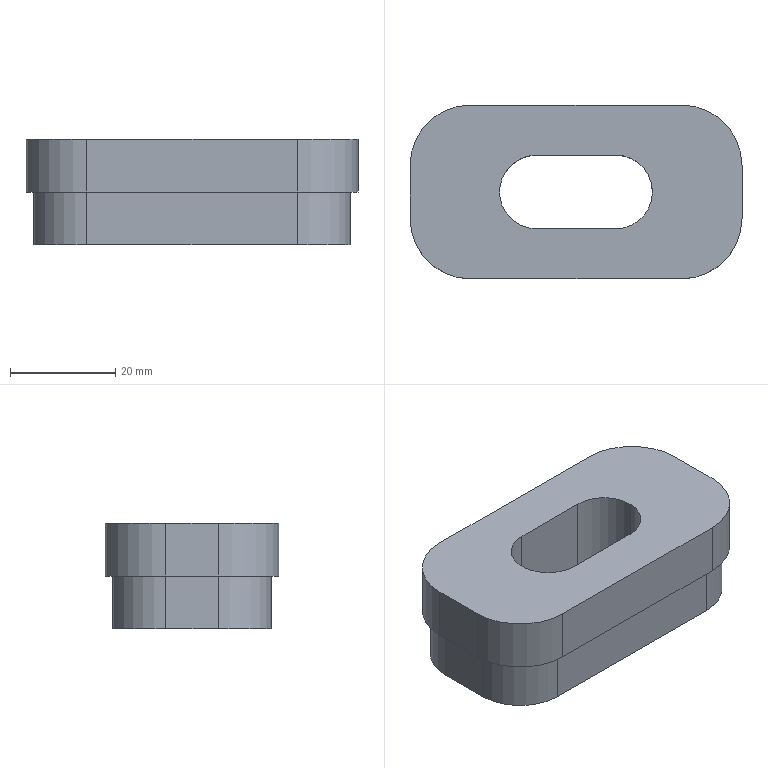Part | SolidWorks | features BaseBody 1 | 1 solid | 24 faces | box 63 x 33 x 20 mm | volume 29518 mm3 | plane 13 | cylinder 11 | commonest cylinder face diameters 20 x4 23 x4 14 x3
STEP:
#1=CARTESIAN_POINT('',(14.5,0.,0.));
#2=VERTEX_POINT('',#1);
#3=CARTESIAN_POINT('',(7.5,7.,0.));
#4=VERTEX_POINT('',#3);
#5=CARTESIAN_POINT('',(7.5,0.,0.));
#6=DIRECTION('',(0.,0.,1.));
#7=DIRECTION('',(1.,0.,0.));
#8=AXIS2_PLACEMENT_3D('',#5,#6,#7);
#9=CIRCLE('',#8,7.);
#10=EDGE_CURVE('',#2,#4,#9,.T.);
#11=ORIENTED_EDGE('',*,*,#10,.F.);
#12=CARTESIAN_POINT('',(14.5,0.,20.));
#13=VERTEX_POINT('',#12);
#14=CARTESIAN_POINT('',(14.5,0.,0.));
#15=DIRECTION('',(0.,0.,1.));
#16=VECTOR('',#15,1000.);
#17=LINE('',#14,#16);
#18=EDGE_CURVE('',#2,#13,#17,.T.);
#19=ORIENTED_EDGE('',*,*,#18,.T.);
#20=CARTESIAN_POINT('',(7.5,7.,20.));
#21=VERTEX_POINT('',#20);
#22=CARTESIAN_POINT('',(7.5,0.,20.));
#23=DIRECTION('',(0.,0.,-1.));
#24=DIRECTION('',(1.,0.,0.));
#25=AXIS2_PLACEMENT_3D('',#22,#23,#24);
#26=CIRCLE('',#25,7.);
#27=EDGE_CURVE('',#21,#13,#26,.T.);
#28=ORIENTED_EDGE('',*,*,#27,.F.);
#29=CARTESIAN_POINT('',(7.5,7.,0.));
#30=DIRECTION('',(0.,0.,1.));
#31=VECTOR('',#30,1000.);
#32=LINE('',#29,#31);
#33=EDGE_CURVE('',#4,#21,#32,.T.);
#34=ORIENTED_EDGE('',*,*,#33,.F.);
#35=EDGE_LOOP('',(#11,#19,#28,#34));
#36=FACE_OUTER_BOUND('',#35,.T.);
#37=CARTESIAN_POINT('',(7.5,0.,0.));
#38=DIRECTION('',(0.,0.,1.));
#39=DIRECTION('',(1.,0.,0.));
#40=AXIS2_PLACEMENT_3D('',#37,#38,#39);
#41=CYLINDRICAL_SURFACE('',#40,7.);
#42=ADVANCED_FACE('',(#36),#41,.F.);
#43=CARTESIAN_POINT('',(7.5,-7.,20.));
#44=VERTEX_POINT('',#43);
#45=CARTESIAN_POINT('',(-7.5,-7.,20.));
#46=VERTEX_POINT('',#45);
#47=CARTESIAN_POINT('',(0.,-7.,20.));
#48=DIRECTION('',(-1.,0.,0.));
#49=VECTOR('',#48,1000.);
#50=LINE('',#47,#49);
#51=EDGE_CURVE('',#44,#46,#50,.T.);
#52=ORIENTED_EDGE('',*,*,#51,.T.);
#53=CARTESIAN_POINT('',(-7.5,7.,20.));
#54=VERTEX_POINT('',#53);
#55=CARTESIAN_POINT('',(-7.5,0.,20.));
#56=DIRECTION('',(0.,0.,-1.));
#57=DIRECTION('',(1.,0.,0.));
#58=AXIS2_PLACEMENT_3D('',#55,#56,#57);
#59=CIRCLE('',#58,7.);
#60=EDGE_CURVE('',#46,#54,#59,.T.);
#61=ORIENTED_EDGE('',*,*,#60,.T.);
#62=CARTESIAN_POINT('',(0.,7.,20.));
#63=DIRECTION('',(1.,0.,0.));
#64=VECTOR('',#63,1000.);
#65=LINE('',#62,#64);
#66=EDGE_CURVE('',#54,#21,#65,.T.);
#67=ORIENTED_EDGE('',*,*,#66,.T.);
#68=ORIENTED_EDGE('',*,*,#27,.T.);
#69=CARTESIAN_POINT('',(7.5,0.,20.));
#70=DIRECTION('',(0.,0.,-1.));
#71=DIRECTION('',(1.,0.,0.));
#72=AXIS2_PLACEMENT_3D('',#69,#70,#71);
#73=CIRCLE('',#72,7.);
#74=EDGE_CURVE('',#13,#44,#73,.T.);
#75=ORIENTED_EDGE('',*,*,#74,.T.);
#76=EDGE_LOOP('',(#52,#61,#67,#68,#75));
#77=FACE_BOUND('',#76,.T.);
#78=CARTESIAN_POINT('',(31.5,-5.,20.));
#79=VERTEX_POINT('',#78);
#80=CARTESIAN_POINT('',(31.5,5.,20.));
#81=VERTEX_POINT('',#80);
#82=CARTESIAN_POINT('',(31.5,0.,20.));
#83=DIRECTION('',(0.,1.,0.));
#84=VECTOR('',#83,1000.);
#85=LINE('',#82,#84);
#86=EDGE_CURVE('',#79,#81,#85,.T.);
#87=ORIENTED_EDGE('',*,*,#86,.T.);
#88=CARTESIAN_POINT('',(20.,16.5,20.));
#89=VERTEX_POINT('',#88);
#90=CARTESIAN_POINT('',(20.,5.,20.));
#91=DIRECTION('',(0.,0.,1.));
#92=DIRECTION('',(1.,0.,0.));
#93=AXIS2_PLACEMENT_3D('',#90,#91,#92);
#94=CIRCLE('',#93,11.5);
#95=EDGE_CURVE('',#81,#89,#94,.T.);
#96=ORIENTED_EDGE('',*,*,#95,.T.);
#97=CARTESIAN_POINT('',(-20.,16.5,20.));
#98=VERTEX_POINT('',#97);
#99=CARTESIAN_POINT('',(0.,16.5,20.));
#100=DIRECTION('',(-1.,0.,0.));
#101=VECTOR('',#100,1000.);
#102=LINE('',#99,#101);
#103=EDGE_CURVE('',#89,#98,#102,.T.);
#104=ORIENTED_EDGE('',*,*,#103,.T.);
#105=CARTESIAN_POINT('',(-31.5,5.,20.));
#106=VERTEX_POINT('',#105);
#107=CARTESIAN_POINT('',(-20.,5.,20.));
#108=DIRECTION('',(0.,0.,1.));
#109=DIRECTION('',(1.,0.,0.));
#110=AXIS2_PLACEMENT_3D('',#107,#108,#109);
#111=CIRCLE('',#110,11.5);
#112=EDGE_CURVE('',#98,#106,#111,.T.);
#113=ORIENTED_EDGE('',*,*,#112,.T.);
#114=CARTESIAN_POINT('',(-31.5,-5.,20.));
#115=VERTEX_POINT('',#114);
#116=CARTESIAN_POINT('',(-31.5,0.,20.));
#117=DIRECTION('',(0.,-1.,0.));
#118=VECTOR('',#117,1000.);
#119=LINE('',#116,#118);
#120=EDGE_CURVE('',#106,#115,#119,.T.);
#121=ORIENTED_EDGE('',*,*,#120,.T.);
#122=CARTESIAN_POINT('',(-20.,-16.5,20.));
#123=VERTEX_POINT('',#122);
#124=CARTESIAN_POINT('',(-20.,-5.,20.));
#125=DIRECTION('',(0.,0.,1.));
#126=DIRECTION('',(1.,0.,0.));
#127=AXIS2_PLACEMENT_3D('',#124,#125,#126);
#128=CIRCLE('',#127,11.5);
#129=EDGE_CURVE('',#115,#123,#128,.T.);
#130=ORIENTED_EDGE('',*,*,#129,.T.);
#131=CARTESIAN_POINT('',(20.,-16.5,20.));
#132=VERTEX_POINT('',#131);
#133=CARTESIAN_POINT('',(0.,-16.5,20.));
#134=DIRECTION('',(1.,0.,0.));
#135=VECTOR('',#134,1000.);
#136=LINE('',#133,#135);
#137=EDGE_CURVE('',#123,#132,#136,.T.);
#138=ORIENTED_EDGE('',*,*,#137,.T.);
#139=CARTESIAN_POINT('',(20.,-5.,20.));
#140=DIRECTION('',(0.,0.,1.));
#141=DIRECTION('',(1.,0.,0.));
#142=AXIS2_PLACEMENT_3D('',#139,#140,#141);
#143=CIRCLE('',#142,11.5);
#144=EDGE_CURVE('',#132,#79,#143,.T.);
#145=ORIENTED_EDGE('',*,*,#144,.T.);
#146=EDGE_LOOP('',(#87,#96,#104,#113,#121,#130,#138,#145));
#147=FACE_OUTER_BOUND('',#146,.T.);
#148=CARTESIAN_POINT('',(0.,0.,20.));
#149=DIRECTION('',(0.,0.,1.));
#150=DIRECTION('',(1.,0.,0.));
#151=AXIS2_PLACEMENT_3D('',#148,#149,#150);
#152=PLANE('',#151);
#153=ADVANCED_FACE('',(#77,#147),#152,.T.);
#154=CARTESIAN_POINT('',(-7.5,7.,0.));
#155=VERTEX_POINT('',#154);
#156=CARTESIAN_POINT('',(-7.5,7.,0.));
#157=DIRECTION('',(0.,0.,-1.));
#158=VECTOR('',#157,1000.);
#159=LINE('',#156,#158);
#160=EDGE_CURVE('',#54,#155,#159,.T.);
#161=ORIENTED_EDGE('',*,*,#160,.F.);
#162=ORIENTED_EDGE('',*,*,#60,.F.);
#163=CARTESIAN_POINT('',(-7.5,-7.,0.));
#164=VERTEX_POINT('',#163);
#165=CARTESIAN_POINT('',(-7.5,-7.,0.));
#166=DIRECTION('',(0.,0.,1.));
#167=VECTOR('',#166,1000.);
#168=LINE('',#165,#167);
#169=EDGE_CURVE('',#164,#46,#168,.T.);
#170=ORIENTED_EDGE('',*,*,#169,.F.);
#171=CARTESIAN_POINT('',(-7.5,0.,0.));
#172=DIRECTION('',(0.,0.,1.));
#173=DIRECTION('',(1.,0.,0.));
#174=AXIS2_PLACEMENT_3D('',#171,#172,#173);
#175=CIRCLE('',#174,7.);
#176=EDGE_CURVE('',#155,#164,#175,.T.);
#177=ORIENTED_EDGE('',*,*,#176,.F.);
#178=EDGE_LOOP('',(#161,#162,#170,#177));
#179=FACE_OUTER_BOUND('',#178,.T.);
#180=CARTESIAN_POINT('',(-7.5,0.,0.));
#181=DIRECTION('',(0.,0.,1.));
#182=DIRECTION('',(1.,0.,0.));
#183=AXIS2_PLACEMENT_3D('',#180,#181,#182);
#184=CYLINDRICAL_SURFACE('',#183,7.);
#185=ADVANCED_FACE('',(#179),#184,.F.);
#186=ORIENTED_EDGE('',*,*,#51,.F.);
#187=CARTESIAN_POINT('',(7.5,-7.,0.));
#188=VERTEX_POINT('',#187);
#189=CARTESIAN_POINT('',(7.5,-7.,9.25));
#190=DIRECTION('',(0.,0.,-1.));
#191=VECTOR('',#190,1000.);
#192=LINE('',#189,#191);
#193=EDGE_CURVE('',#44,#188,#192,.T.);
#194=ORIENTED_EDGE('',*,*,#193,.T.);
#195=CARTESIAN_POINT('',(0.,-7.,0.));
#196=DIRECTION('',(-1.,0.,0.));
#197=VECTOR('',#196,1000.);
#198=LINE('',#195,#197);
#199=EDGE_CURVE('',#188,#164,#198,.T.);
#200=ORIENTED_EDGE('',*,*,#199,.T.);
#201=ORIENTED_EDGE('',*,*,#169,.T.);
#202=EDGE_LOOP('',(#186,#194,#200,#201));
#203=FACE_OUTER_BOUND('',#202,.T.);
#204=CARTESIAN_POINT('',(0.,-7.,9.25));
#205=DIRECTION('',(0.,1.,0.));
#206=DIRECTION('',(0.,0.,1.));
#207=AXIS2_PLACEMENT_3D('',#204,#205,#206);
#208=PLANE('',#207);
#209=ADVANCED_FACE('',(#203),#208,.T.);
#210=ORIENTED_EDGE('',*,*,#18,.F.);
#211=CARTESIAN_POINT('',(7.5,0.,0.));
#212=DIRECTION('',(0.,0.,1.));
#213=DIRECTION('',(1.,0.,0.));
#214=AXIS2_PLACEMENT_3D('',#211,#212,#213);
#215=CIRCLE('',#214,7.);
#216=EDGE_CURVE('',#188,#2,#215,.T.);
#217=ORIENTED_EDGE('',*,*,#216,.F.);
#218=ORIENTED_EDGE('',*,*,#193,.F.);
#219=ORIENTED_EDGE('',*,*,#74,.F.);
#220=EDGE_LOOP('',(#210,#217,#218,#219));
#221=FACE_OUTER_BOUND('',#220,.T.);
#222=CARTESIAN_POINT('',(7.5,0.,0.));
#223=DIRECTION('',(0.,0.,1.));
#224=DIRECTION('',(1.,0.,0.));
#225=AXIS2_PLACEMENT_3D('',#222,#223,#224);
#226=CYLINDRICAL_SURFACE('',#225,7.);
#227=ADVANCED_FACE('',(#221),#226,.F.);
#228=ORIENTED_EDGE('',*,*,#33,.T.);
#229=ORIENTED_EDGE('',*,*,#66,.F.);
#230=ORIENTED_EDGE('',*,*,#160,.T.);
#231=CARTESIAN_POINT('',(0.,7.,0.));
#232=DIRECTION('',(-1.,0.,0.));
#233=VECTOR('',#232,1000.);
#234=LINE('',#231,#233);
#235=EDGE_CURVE('',#4,#155,#234,.T.);
#236=ORIENTED_EDGE('',*,*,#235,.F.);
#237=EDGE_LOOP('',(#228,#229,#230,#236));
#238=FACE_OUTER_BOUND('',#237,.T.);
#239=CARTESIAN_POINT('',(0.,7.,9.25));
#240=DIRECTION('',(0.,1.,0.));
#241=DIRECTION('',(0.,0.,1.));
#242=AXIS2_PLACEMENT_3D('',#239,#240,#241);
#243=PLANE('',#242);
#244=ADVANCED_FACE('',(#238),#243,.F.);
#245=CARTESIAN_POINT('',(20.,16.5,10.));
#246=VERTEX_POINT('',#245);
#247=CARTESIAN_POINT('',(20.,16.5,10.));
#248=DIRECTION('',(0.,0.,1.));
#249=VECTOR('',#248,1000.);
#250=LINE('',#247,#249);
#251=EDGE_CURVE('',#246,#89,#250,.T.);
#252=ORIENTED_EDGE('',*,*,#251,.T.);
#253=ORIENTED_EDGE('',*,*,#95,.F.);
#254=CARTESIAN_POINT('',(31.5,5.,10.));
#255=VERTEX_POINT('',#254);
#256=CARTESIAN_POINT('',(31.5,5.,10.));
#257=DIRECTION('',(0.,0.,-1.));
#258=VECTOR('',#257,1000.);
#259=LINE('',#256,#258);
#260=EDGE_CURVE('',#81,#255,#259,.T.);
#261=ORIENTED_EDGE('',*,*,#260,.T.);
#262=CARTESIAN_POINT('',(20.,5.,10.));
#263=DIRECTION('',(0.,0.,1.));
#264=DIRECTION('',(1.,0.,0.));
#265=AXIS2_PLACEMENT_3D('',#262,#263,#264);
#266=CIRCLE('',#265,11.5);
#267=EDGE_CURVE('',#255,#246,#266,.T.);
#268=ORIENTED_EDGE('',*,*,#267,.T.);
#269=EDGE_LOOP('',(#252,#253,#261,#268));
#270=FACE_OUTER_BOUND('',#269,.T.);
#271=CARTESIAN_POINT('',(20.,5.,10.));
#272=DIRECTION('',(0.,0.,1.));
#273=DIRECTION('',(1.,0.,0.));
#274=AXIS2_PLACEMENT_3D('',#271,#272,#273);
#275=CYLINDRICAL_SURFACE('',#274,11.5);
#276=ADVANCED_FACE('',(#270),#275,.T.);
#277=ORIENTED_EDGE('',*,*,#260,.F.);
#278=ORIENTED_EDGE('',*,*,#86,.F.);
#279=CARTESIAN_POINT('',(31.5,-5.,10.));
#280=VERTEX_POINT('',#279);
#281=CARTESIAN_POINT('',(31.5,-5.,15.));
#282=DIRECTION('',(0.,0.,-1.));
#283=VECTOR('',#282,1000.);
#284=LINE('',#281,#283);
#285=EDGE_CURVE('',#79,#280,#284,.T.);
#286=ORIENTED_EDGE('',*,*,#285,.T.);
#287=CARTESIAN_POINT('',(31.5,0.,10.));
#288=DIRECTION('',(0.,1.,0.));
#289=VECTOR('',#288,1000.);
#290=LINE('',#287,#289);
#291=EDGE_CURVE('',#280,#255,#290,.T.);
#292=ORIENTED_EDGE('',*,*,#291,.T.);
#293=EDGE_LOOP('',(#277,#278,#286,#292));
#294=FACE_OUTER_BOUND('',#293,.T.);
#295=CARTESIAN_POINT('',(31.5,0.,15.));
#296=DIRECTION('',(1.,0.,0.));
#297=DIRECTION('',(0.,0.,-1.));
#298=AXIS2_PLACEMENT_3D('',#295,#296,#297);
#299=PLANE('',#298);
#300=ADVANCED_FACE('',(#294),#299,.T.);
#301=ORIENTED_EDGE('',*,*,#285,.F.);
#302=ORIENTED_EDGE('',*,*,#144,.F.);
#303=CARTESIAN_POINT('',(20.,-16.5,10.));
#304=VERTEX_POINT('',#303);
#305=CARTESIAN_POINT('',(20.,-16.5,10.));
#306=DIRECTION('',(0.,0.,-1.));
#307=VECTOR('',#306,1000.);
#308=LINE('',#305,#307);
#309=EDGE_CURVE('',#132,#304,#308,.T.);
#310=ORIENTED_EDGE('',*,*,#309,.T.);
#311=CARTESIAN_POINT('',(20.,-5.,10.));
#312=DIRECTION('',(0.,0.,1.));
#313=DIRECTION('',(1.,0.,0.));
#314=AXIS2_PLACEMENT_3D('',#311,#312,#313);
#315=CIRCLE('',#314,11.5);
#316=EDGE_CURVE('',#304,#280,#315,.T.);
#317=ORIENTED_EDGE('',*,*,#316,.T.);
#318=EDGE_LOOP('',(#301,#302,#310,#317));
#319=FACE_OUTER_BOUND('',#318,.T.);
#320=CARTESIAN_POINT('',(20.,-5.,10.));
#321=DIRECTION('',(0.,0.,1.));
#322=DIRECTION('',(1.,0.,0.));
#323=AXIS2_PLACEMENT_3D('',#320,#321,#322);
#324=CYLINDRICAL_SURFACE('',#323,11.5);
#325=ADVANCED_FACE('',(#319),#324,.T.);
#326=CARTESIAN_POINT('',(-20.,-16.5,10.));
#327=VERTEX_POINT('',#326);
#328=CARTESIAN_POINT('',(0.,-16.5,10.));
#329=DIRECTION('',(-1.,0.,0.));
#330=VECTOR('',#329,1000.);
#331=LINE('',#328,#330);
#332=EDGE_CURVE('',#304,#327,#331,.T.);
#333=ORIENTED_EDGE('',*,*,#332,.F.);
#334=ORIENTED_EDGE('',*,*,#309,.F.);
#335=ORIENTED_EDGE('',*,*,#137,.F.);
#336=CARTESIAN_POINT('',(-20.,-16.5,15.));
#337=DIRECTION('',(0.,0.,1.));
#338=VECTOR('',#337,1000.);
#339=LINE('',#336,#338);
#340=EDGE_CURVE('',#327,#123,#339,.T.);
#341=ORIENTED_EDGE('',*,*,#340,.F.);
#342=EDGE_LOOP('',(#333,#334,#335,#341));
#343=FACE_OUTER_BOUND('',#342,.T.);
#344=CARTESIAN_POINT('',(0.,-16.5,15.));
#345=DIRECTION('',(0.,1.,0.));
#346=DIRECTION('',(0.,0.,1.));
#347=AXIS2_PLACEMENT_3D('',#344,#345,#346);
#348=PLANE('',#347);
#349=ADVANCED_FACE('',(#343),#348,.F.);
#350=ORIENTED_EDGE('',*,*,#340,.T.);
#351=ORIENTED_EDGE('',*,*,#129,.F.);
#352=CARTESIAN_POINT('',(-31.5,-5.,10.));
#353=VERTEX_POINT('',#352);
#354=CARTESIAN_POINT('',(-31.5,-5.,10.));
#355=DIRECTION('',(0.,0.,-1.));
#356=VECTOR('',#355,1000.);
#357=LINE('',#354,#356);
#358=EDGE_CURVE('',#115,#353,#357,.T.);
#359=ORIENTED_EDGE('',*,*,#358,.T.);
#360=CARTESIAN_POINT('',(-20.,-5.,10.));
#361=DIRECTION('',(0.,0.,1.));
#362=DIRECTION('',(1.,0.,0.));
#363=AXIS2_PLACEMENT_3D('',#360,#361,#362);
#364=CIRCLE('',#363,11.5);
#365=EDGE_CURVE('',#353,#327,#364,.T.);
#366=ORIENTED_EDGE('',*,*,#365,.T.);
#367=EDGE_LOOP('',(#350,#351,#359,#366));
#368=FACE_OUTER_BOUND('',#367,.T.);
#369=CARTESIAN_POINT('',(-20.,-5.,10.));
#370=DIRECTION('',(0.,0.,1.));
#371=DIRECTION('',(1.,0.,0.));
#372=AXIS2_PLACEMENT_3D('',#369,#370,#371);
#373=CYLINDRICAL_SURFACE('',#372,11.5);
#374=ADVANCED_FACE('',(#368),#373,.T.);
#375=CARTESIAN_POINT('',(-31.5,5.,10.));
#376=VERTEX_POINT('',#375);
#377=CARTESIAN_POINT('',(-31.5,0.,10.));
#378=DIRECTION('',(0.,1.,0.));
#379=VECTOR('',#378,1000.);
#380=LINE('',#377,#379);
#381=EDGE_CURVE('',#353,#376,#380,.T.);
#382=ORIENTED_EDGE('',*,*,#381,.F.);
#383=ORIENTED_EDGE('',*,*,#358,.F.);
#384=ORIENTED_EDGE('',*,*,#120,.F.);
#385=CARTESIAN_POINT('',(-31.5,5.,15.));
#386=DIRECTION('',(0.,0.,1.));
#387=VECTOR('',#386,1000.);
#388=LINE('',#385,#387);
#389=EDGE_CURVE('',#376,#106,#388,.T.);
#390=ORIENTED_EDGE('',*,*,#389,.F.);
#391=EDGE_LOOP('',(#382,#383,#384,#390));
#392=FACE_OUTER_BOUND('',#391,.T.);
#393=CARTESIAN_POINT('',(-31.5,0.,15.));
#394=DIRECTION('',(1.,0.,0.));
#395=DIRECTION('',(0.,0.,-1.));
#396=AXIS2_PLACEMENT_3D('',#393,#394,#395);
#397=PLANE('',#396);
#398=ADVANCED_FACE('',(#392),#397,.F.);
#399=ORIENTED_EDGE('',*,*,#389,.T.);
#400=ORIENTED_EDGE('',*,*,#112,.F.);
#401=CARTESIAN_POINT('',(-20.,16.5,10.));
#402=VERTEX_POINT('',#401);
#403=CARTESIAN_POINT('',(-20.,16.5,10.));
#404=DIRECTION('',(0.,0.,-1.));
#405=VECTOR('',#404,1000.);
#406=LINE('',#403,#405);
#407=EDGE_CURVE('',#98,#402,#406,.T.);
#408=ORIENTED_EDGE('',*,*,#407,.T.);
#409=CARTESIAN_POINT('',(-20.,5.,10.));
#410=DIRECTION('',(0.,0.,1.));
#411=DIRECTION('',(1.,0.,0.));
#412=AXIS2_PLACEMENT_3D('',#409,#410,#411);
#413=CIRCLE('',#412,11.5);
#414=EDGE_CURVE('',#402,#376,#413,.T.);
#415=ORIENTED_EDGE('',*,*,#414,.T.);
#416=EDGE_LOOP('',(#399,#400,#408,#415));
#417=FACE_OUTER_BOUND('',#416,.T.);
#418=CARTESIAN_POINT('',(-20.,5.,10.));
#419=DIRECTION('',(0.,0.,1.));
#420=DIRECTION('',(1.,0.,0.));
#421=AXIS2_PLACEMENT_3D('',#418,#419,#420);
#422=CYLINDRICAL_SURFACE('',#421,11.5);
#423=ADVANCED_FACE('',(#417),#422,.T.);
#424=ORIENTED_EDGE('',*,*,#407,.F.);
#425=ORIENTED_EDGE('',*,*,#103,.F.);
#426=ORIENTED_EDGE('',*,*,#251,.F.);
#427=CARTESIAN_POINT('',(0.,16.5,10.));
#428=DIRECTION('',(-1.,0.,0.));
#429=VECTOR('',#428,1000.);
#430=LINE('',#427,#429);
#431=EDGE_CURVE('',#246,#402,#430,.T.);
#432=ORIENTED_EDGE('',*,*,#431,.T.);
#433=EDGE_LOOP('',(#424,#425,#426,#432));
#434=FACE_OUTER_BOUND('',#433,.T.);
#435=CARTESIAN_POINT('',(0.,16.5,15.));
#436=DIRECTION('',(0.,1.,0.));
#437=DIRECTION('',(0.,0.,1.));
#438=AXIS2_PLACEMENT_3D('',#435,#436,#437);
#439=PLANE('',#438);
#440=ADVANCED_FACE('',(#434),#439,.T.);
#441=ORIENTED_EDGE('',*,*,#216,.T.);
#442=ORIENTED_EDGE('',*,*,#10,.T.);
#443=ORIENTED_EDGE('',*,*,#235,.T.);
#444=ORIENTED_EDGE('',*,*,#176,.T.);
#445=ORIENTED_EDGE('',*,*,#199,.F.);
#446=EDGE_LOOP('',(#441,#442,#443,#444,#445));
#447=FACE_BOUND('',#446,.T.);
#448=CARTESIAN_POINT('',(20.,-15.,0.));
#449=VERTEX_POINT('',#448);
#450=CARTESIAN_POINT('',(30.,-5.,0.));
#451=VERTEX_POINT('',#450);
#452=CARTESIAN_POINT('',(20.,-5.,0.));
#453=DIRECTION('',(0.,0.,1.));
#454=DIRECTION('',(-1.,0.,0.));
#455=AXIS2_PLACEMENT_3D('',#452,#453,#454);
#456=CIRCLE('',#455,10.);
#457=EDGE_CURVE('',#449,#451,#456,.T.);
#458=ORIENTED_EDGE('',*,*,#457,.F.);
#459=CARTESIAN_POINT('',(-20.,-15.,0.));
#460=VERTEX_POINT('',#459);
#461=CARTESIAN_POINT('',(0.,-15.,0.));
#462=DIRECTION('',(1.,0.,0.));
#463=VECTOR('',#462,1000.);
#464=LINE('',#461,#463);
#465=EDGE_CURVE('',#460,#449,#464,.T.);
#466=ORIENTED_EDGE('',*,*,#465,.F.);
#467=CARTESIAN_POINT('',(-30.,-5.,0.));
#468=VERTEX_POINT('',#467);
#469=CARTESIAN_POINT('',(-20.,-5.,0.));
#470=DIRECTION('',(0.,0.,1.));
#471=DIRECTION('',(-1.,0.,0.));
#472=AXIS2_PLACEMENT_3D('',#469,#470,#471);
#473=CIRCLE('',#472,10.);
#474=EDGE_CURVE('',#468,#460,#473,.T.);
#475=ORIENTED_EDGE('',*,*,#474,.F.);
#476=CARTESIAN_POINT('',(-30.,5.,0.));
#477=VERTEX_POINT('',#476);
#478=CARTESIAN_POINT('',(-30.,0.,0.));
#479=DIRECTION('',(0.,-1.,0.));
#480=VECTOR('',#479,1000.);
#481=LINE('',#478,#480);
#482=EDGE_CURVE('',#477,#468,#481,.T.);
#483=ORIENTED_EDGE('',*,*,#482,.F.);
#484=CARTESIAN_POINT('',(-20.,15.,0.));
#485=VERTEX_POINT('',#484);
#486=CARTESIAN_POINT('',(-20.,5.,0.));
#487=DIRECTION('',(0.,0.,1.));
#488=DIRECTION('',(-1.,0.,0.));
#489=AXIS2_PLACEMENT_3D('',#486,#487,#488);
#490=CIRCLE('',#489,10.);
#491=EDGE_CURVE('',#485,#477,#490,.T.);
#492=ORIENTED_EDGE('',*,*,#491,.F.);
#493=CARTESIAN_POINT('',(20.,15.,0.));
#494=VERTEX_POINT('',#493);
#495=CARTESIAN_POINT('',(0.,15.,0.));
#496=DIRECTION('',(-1.,0.,0.));
#497=VECTOR('',#496,1000.);
#498=LINE('',#495,#497);
#499=EDGE_CURVE('',#494,#485,#498,.T.);
#500=ORIENTED_EDGE('',*,*,#499,.F.);
#501=CARTESIAN_POINT('',(30.,5.,0.));
#502=VERTEX_POINT('',#501);
#503=CARTESIAN_POINT('',(20.,5.,0.));
#504=DIRECTION('',(0.,0.,1.));
#505=DIRECTION('',(-1.,0.,0.));
#506=AXIS2_PLACEMENT_3D('',#503,#504,#505);
#507=CIRCLE('',#506,10.);
#508=EDGE_CURVE('',#502,#494,#507,.T.);
#509=ORIENTED_EDGE('',*,*,#508,.F.);
#510=CARTESIAN_POINT('',(30.,0.,0.));
#511=DIRECTION('',(0.,1.,0.));
#512=VECTOR('',#511,1000.);
#513=LINE('',#510,#512);
#514=EDGE_CURVE('',#451,#502,#513,.T.);
#515=ORIENTED_EDGE('',*,*,#514,.F.);
#516=EDGE_LOOP('',(#458,#466,#475,#483,#492,#500,#509,#515));
#517=FACE_OUTER_BOUND('',#516,.T.);
#518=CARTESIAN_POINT('',(0.,0.,0.));
#519=DIRECTION('',(0.,0.,1.));
#520=DIRECTION('',(1.,0.,0.));
#521=AXIS2_PLACEMENT_3D('',#518,#519,#520);
#522=PLANE('',#521);
#523=ADVANCED_FACE('',(#447,#517),#522,.F.);
#524=CARTESIAN_POINT('',(-30.,5.,10.));
#525=VERTEX_POINT('',#524);
#526=CARTESIAN_POINT('',(-20.,15.,10.));
#527=VERTEX_POINT('',#526);
#528=CARTESIAN_POINT('',(-20.,5.,10.));
#529=DIRECTION('',(0.,0.,-1.));
#530=DIRECTION('',(-1.,0.,0.));
#531=AXIS2_PLACEMENT_3D('',#528,#529,#530);
#532=CIRCLE('',#531,10.);
#533=EDGE_CURVE('',#525,#527,#532,.T.);
#534=ORIENTED_EDGE('',*,*,#533,.F.);
#535=CARTESIAN_POINT('',(-30.,-5.,10.));
#536=VERTEX_POINT('',#535);
#537=CARTESIAN_POINT('',(-30.,0.,10.));
#538=DIRECTION('',(0.,1.,0.));
#539=VECTOR('',#538,1000.);
#540=LINE('',#537,#539);
#541=EDGE_CURVE('',#536,#525,#540,.T.);
#542=ORIENTED_EDGE('',*,*,#541,.F.);
#543=CARTESIAN_POINT('',(-20.,-15.,10.));
#544=VERTEX_POINT('',#543);
#545=CARTESIAN_POINT('',(-20.,-5.,10.));
#546=DIRECTION('',(0.,0.,-1.));
#547=DIRECTION('',(-1.,0.,0.));
#548=AXIS2_PLACEMENT_3D('',#545,#546,#547);
#549=CIRCLE('',#548,10.);
#550=EDGE_CURVE('',#544,#536,#549,.T.);
#551=ORIENTED_EDGE('',*,*,#550,.F.);
#552=CARTESIAN_POINT('',(20.,-15.,10.));
#553=VERTEX_POINT('',#552);
#554=CARTESIAN_POINT('',(0.,-15.,10.));
#555=DIRECTION('',(-1.,0.,0.));
#556=VECTOR('',#555,1000.);
#557=LINE('',#554,#556);
#558=EDGE_CURVE('',#553,#544,#557,.T.);
#559=ORIENTED_EDGE('',*,*,#558,.F.);
#560=CARTESIAN_POINT('',(30.,-5.,10.));
#561=VERTEX_POINT('',#560);
#562=CARTESIAN_POINT('',(20.,-5.,10.));
#563=DIRECTION('',(0.,0.,-1.));
#564=DIRECTION('',(-1.,0.,0.));
#565=AXIS2_PLACEMENT_3D('',#562,#563,#564);
#566=CIRCLE('',#565,10.);
#567=EDGE_CURVE('',#561,#553,#566,.T.);
#568=ORIENTED_EDGE('',*,*,#567,.F.);
#569=CARTESIAN_POINT('',(30.,5.,10.));
#570=VERTEX_POINT('',#569);
#571=CARTESIAN_POINT('',(30.,0.,10.));
#572=DIRECTION('',(0.,-1.,0.));
#573=VECTOR('',#572,1000.);
#574=LINE('',#571,#573);
#575=EDGE_CURVE('',#570,#561,#574,.T.);
#576=ORIENTED_EDGE('',*,*,#575,.F.);
#577=CARTESIAN_POINT('',(20.,15.,10.));
#578=VERTEX_POINT('',#577);
#579=CARTESIAN_POINT('',(20.,5.,10.));
#580=DIRECTION('',(0.,0.,-1.));
#581=DIRECTION('',(-1.,0.,0.));
#582=AXIS2_PLACEMENT_3D('',#579,#580,#581);
#583=CIRCLE('',#582,10.);
#584=EDGE_CURVE('',#578,#570,#583,.T.);
#585=ORIENTED_EDGE('',*,*,#584,.F.);
#586=CARTESIAN_POINT('',(0.,15.,10.));
#587=DIRECTION('',(1.,0.,0.));
#588=VECTOR('',#587,1000.);
#589=LINE('',#586,#588);
#590=EDGE_CURVE('',#527,#578,#589,.T.);
#591=ORIENTED_EDGE('',*,*,#590,.F.);
#592=EDGE_LOOP('',(#534,#542,#551,#559,#568,#576,#585,#591));
#593=FACE_BOUND('',#592,.T.);
#594=ORIENTED_EDGE('',*,*,#291,.F.);
#595=ORIENTED_EDGE('',*,*,#316,.F.);
#596=ORIENTED_EDGE('',*,*,#332,.T.);
#597=ORIENTED_EDGE('',*,*,#365,.F.);
#598=ORIENTED_EDGE('',*,*,#381,.T.);
#599=ORIENTED_EDGE('',*,*,#414,.F.);
#600=ORIENTED_EDGE('',*,*,#431,.F.);
#601=ORIENTED_EDGE('',*,*,#267,.F.);
#602=EDGE_LOOP('',(#594,#595,#596,#597,#598,#599,#600,#601));
#603=FACE_OUTER_BOUND('',#602,.T.);
#604=CARTESIAN_POINT('',(0.,0.,10.));
#605=DIRECTION('',(0.,0.,1.));
#606=DIRECTION('',(1.,0.,0.));
#607=AXIS2_PLACEMENT_3D('',#604,#605,#606);
#608=PLANE('',#607);
#609=ADVANCED_FACE('',(#593,#603),#608,.F.);
#610=CARTESIAN_POINT('',(30.,5.,9.25));
#611=DIRECTION('',(0.,0.,1.));
#612=VECTOR('',#611,1000.);
#613=LINE('',#610,#612);
#614=EDGE_CURVE('',#502,#570,#613,.T.);
#615=ORIENTED_EDGE('',*,*,#614,.T.);
#616=ORIENTED_EDGE('',*,*,#575,.T.);
#617=CARTESIAN_POINT('',(30.,-5.,9.25));
#618=DIRECTION('',(0.,0.,-1.));
#619=VECTOR('',#618,1000.);
#620=LINE('',#617,#619);
#621=EDGE_CURVE('',#561,#451,#620,.T.);
#622=ORIENTED_EDGE('',*,*,#621,.T.);
#623=ORIENTED_EDGE('',*,*,#514,.T.);
#624=EDGE_LOOP('',(#615,#616,#622,#623));
#625=FACE_OUTER_BOUND('',#624,.T.);
#626=CARTESIAN_POINT('',(30.,0.,9.25));
#627=DIRECTION('',(1.,0.,0.));
#628=DIRECTION('',(0.,0.,-1.));
#629=AXIS2_PLACEMENT_3D('',#626,#627,#628);
#630=PLANE('',#629);
#631=ADVANCED_FACE('',(#625),#630,.T.);
#632=ORIENTED_EDGE('',*,*,#621,.F.);
#633=ORIENTED_EDGE('',*,*,#567,.T.);
#634=CARTESIAN_POINT('',(20.,-15.,18.5));
#635=DIRECTION('',(0.,0.,-1.));
#636=VECTOR('',#635,1000.);
#637=LINE('',#634,#636);
#638=EDGE_CURVE('',#553,#449,#637,.T.);
#639=ORIENTED_EDGE('',*,*,#638,.T.);
#640=ORIENTED_EDGE('',*,*,#457,.T.);
#641=EDGE_LOOP('',(#632,#633,#639,#640));
#642=FACE_OUTER_BOUND('',#641,.T.);
#643=CARTESIAN_POINT('',(20.,-5.,18.5));
#644=DIRECTION('',(0.,0.,-1.));
#645=DIRECTION('',(-1.,0.,0.));
#646=AXIS2_PLACEMENT_3D('',#643,#644,#645);
#647=CYLINDRICAL_SURFACE('',#646,10.);
#648=ADVANCED_FACE('',(#642),#647,.T.);
#649=ORIENTED_EDGE('',*,*,#465,.T.);
#650=ORIENTED_EDGE('',*,*,#638,.F.);
#651=ORIENTED_EDGE('',*,*,#558,.T.);
#652=CARTESIAN_POINT('',(-20.,-15.,9.25));
#653=DIRECTION('',(0.,0.,1.));
#654=VECTOR('',#653,1000.);
#655=LINE('',#652,#654);
#656=EDGE_CURVE('',#460,#544,#655,.T.);
#657=ORIENTED_EDGE('',*,*,#656,.F.);
#658=EDGE_LOOP('',(#649,#650,#651,#657));
#659=FACE_OUTER_BOUND('',#658,.T.);
#660=CARTESIAN_POINT('',(0.,-15.,9.25));
#661=DIRECTION('',(0.,1.,0.));
#662=DIRECTION('',(0.,0.,1.));
#663=AXIS2_PLACEMENT_3D('',#660,#661,#662);
#664=PLANE('',#663);
#665=ADVANCED_FACE('',(#659),#664,.F.);
#666=ORIENTED_EDGE('',*,*,#656,.T.);
#667=ORIENTED_EDGE('',*,*,#550,.T.);
#668=CARTESIAN_POINT('',(-30.,-5.,9.25));
#669=DIRECTION('',(0.,0.,-1.));
#670=VECTOR('',#669,1000.);
#671=LINE('',#668,#670);
#672=EDGE_CURVE('',#536,#468,#671,.T.);
#673=ORIENTED_EDGE('',*,*,#672,.T.);
#674=ORIENTED_EDGE('',*,*,#474,.T.);
#675=EDGE_LOOP('',(#666,#667,#673,#674));
#676=FACE_OUTER_BOUND('',#675,.T.);
#677=CARTESIAN_POINT('',(-20.,-5.,18.5));
#678=DIRECTION('',(0.,0.,-1.));
#679=DIRECTION('',(-1.,0.,0.));
#680=AXIS2_PLACEMENT_3D('',#677,#678,#679);
#681=CYLINDRICAL_SURFACE('',#680,10.);
#682=ADVANCED_FACE('',(#676),#681,.T.);
#683=ORIENTED_EDGE('',*,*,#482,.T.);
#684=ORIENTED_EDGE('',*,*,#672,.F.);
#685=ORIENTED_EDGE('',*,*,#541,.T.);
#686=CARTESIAN_POINT('',(-30.,5.,9.25));
#687=DIRECTION('',(0.,0.,1.));
#688=VECTOR('',#687,1000.);
#689=LINE('',#686,#688);
#690=EDGE_CURVE('',#477,#525,#689,.T.);
#691=ORIENTED_EDGE('',*,*,#690,.F.);
#692=EDGE_LOOP('',(#683,#684,#685,#691));
#693=FACE_OUTER_BOUND('',#692,.T.);
#694=CARTESIAN_POINT('',(-30.,0.,9.25));
#695=DIRECTION('',(1.,0.,0.));
#696=DIRECTION('',(0.,0.,-1.));
#697=AXIS2_PLACEMENT_3D('',#694,#695,#696);
#698=PLANE('',#697);
#699=ADVANCED_FACE('',(#693),#698,.F.);
#700=ORIENTED_EDGE('',*,*,#690,.T.);
#701=ORIENTED_EDGE('',*,*,#533,.T.);
#702=CARTESIAN_POINT('',(-20.,15.,18.5));
#703=DIRECTION('',(0.,0.,-1.));
#704=VECTOR('',#703,1000.);
#705=LINE('',#702,#704);
#706=EDGE_CURVE('',#527,#485,#705,.T.);
#707=ORIENTED_EDGE('',*,*,#706,.T.);
#708=ORIENTED_EDGE('',*,*,#491,.T.);
#709=EDGE_LOOP('',(#700,#701,#707,#708));
#710=FACE_OUTER_BOUND('',#709,.T.);
#711=CARTESIAN_POINT('',(-20.,5.,18.5));
#712=DIRECTION('',(0.,0.,-1.));
#713=DIRECTION('',(-1.,0.,0.));
#714=AXIS2_PLACEMENT_3D('',#711,#712,#713);
#715=CYLINDRICAL_SURFACE('',#714,10.);
#716=ADVANCED_FACE('',(#710),#715,.T.);
#717=ORIENTED_EDGE('',*,*,#706,.F.);
#718=ORIENTED_EDGE('',*,*,#590,.T.);
#719=CARTESIAN_POINT('',(20.,15.,9.25));
#720=DIRECTION('',(0.,0.,-1.));
#721=VECTOR('',#720,1000.);
#722=LINE('',#719,#721);
#723=EDGE_CURVE('',#578,#494,#722,.T.);
#724=ORIENTED_EDGE('',*,*,#723,.T.);
#725=ORIENTED_EDGE('',*,*,#499,.T.);
#726=EDGE_LOOP('',(#717,#718,#724,#725));
#727=FACE_OUTER_BOUND('',#726,.T.);
#728=CARTESIAN_POINT('',(0.,15.,9.25));
#729=DIRECTION('',(0.,1.,0.));
#730=DIRECTION('',(0.,0.,1.));
#731=AXIS2_PLACEMENT_3D('',#728,#729,#730);
#732=PLANE('',#731);
#733=ADVANCED_FACE('',(#727),#732,.T.);
#734=ORIENTED_EDGE('',*,*,#723,.F.);
#735=ORIENTED_EDGE('',*,*,#584,.T.);
#736=ORIENTED_EDGE('',*,*,#614,.F.);
#737=ORIENTED_EDGE('',*,*,#508,.T.);
#738=EDGE_LOOP('',(#734,#735,#736,#737));
#739=FACE_OUTER_BOUND('',#738,.T.);
#740=CARTESIAN_POINT('',(20.,5.,18.5));
#741=DIRECTION('',(0.,0.,-1.));
#742=DIRECTION('',(-1.,0.,0.));
#743=AXIS2_PLACEMENT_3D('',#740,#741,#742);
#744=CYLINDRICAL_SURFACE('',#743,10.);
#745=ADVANCED_FACE('',(#739),#744,.T.);
#746=CLOSED_SHELL('',(#42,#153,#185,#209,#227,#244,#276,#300,#325,#349,#374,#398,#423,#440,#523,#609,#631,#648,#665,#682,#699,#716,#733,#745));
#747=MANIFOLD_SOLID_BREP('',#746);
#748=CARTESIAN_POINT('',(0.,0.,0.));
#749=DIRECTION('',(0.,0.,1.));
#750=DIRECTION('',(1.,0.,0.));
#751=AXIS2_PLACEMENT_3D('',#748,#749,#750);
#752=(LENGTH_UNIT()NAMED_UNIT(*)SI_UNIT(.MILLI.,.METRE.));
#753=UNCERTAINTY_MEASURE_WITH_UNIT(LENGTH_MEASURE(0.00001),#752,'','');
#754=(NAMED_UNIT(*)PLANE_ANGLE_UNIT()SI_UNIT($,.RADIAN.));
#755=(NAMED_UNIT(*)SI_UNIT($,.STERADIAN.)SOLID_ANGLE_UNIT());
#756=(GEOMETRIC_REPRESENTATION_CONTEXT(3)GLOBAL_UNCERTAINTY_ASSIGNED_CONTEXT((#753))GLOBAL_UNIT_ASSIGNED_CONTEXT((#752,#754,#755))REPRESENTATION_CONTEXT('',''));
#757=ADVANCED_BREP_SHAPE_REPRESENTATION('',(#747,#751),#756);